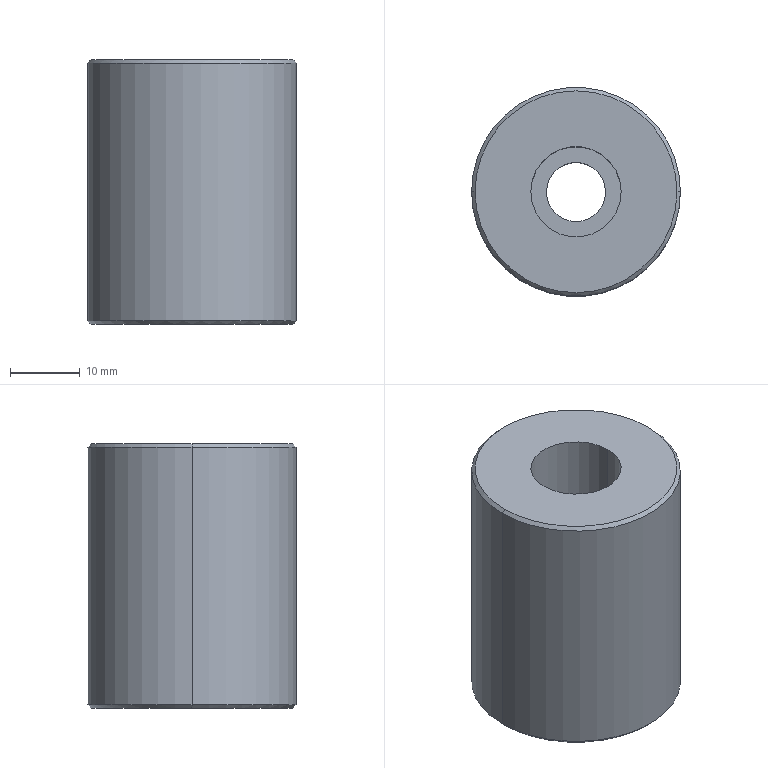Part | STEP file | PN_0003 Press shell nylon post | 1 solid | 13 faces | box 30 x 30 x 38 mm | volume 22857 mm3 | cylinder 6 | cone 4 | plane 3 | commonest cylinder face diameters 8.5 x2 13 x2 30 x2
STEP:
#1=CARTESIAN_POINT('',(0.,0.,0.));
#2=DIRECTION('',(0.,0.,1.));
#3=DIRECTION('',(1.,0.,0.));
#4=AXIS2_PLACEMENT_3D('',#1,#2,#3);
#5=CARTESIAN_POINT('',(14.5,0.,19.));
#6=VERTEX_POINT('',#5);
#7=CARTESIAN_POINT('',(-14.5,0.,19.));
#8=VERTEX_POINT('',#7);
#9=CARTESIAN_POINT('',(0.,0.,19.));
#10=DIRECTION('',(0.,0.,1.));
#11=DIRECTION('',(1.,0.,0.));
#12=AXIS2_PLACEMENT_3D('',#9,#10,#11);
#13=CIRCLE('',#12,14.5);
#14=CARTESIAN_POINT('',(0.,0.,19.));
#15=DIRECTION('',(0.,0.,-1.));
#16=DIRECTION('',(-1.,0.,0.));
#17=AXIS2_PLACEMENT_3D('',#14,#15,#16);
#18=CONICAL_SURFACE('',#17,14.5,0.7854);
#19=CARTESIAN_POINT('',(3.142,0.));
#20=DIRECTION('',(-1.,0.));
#21=VECTOR('',#20,1.);
#22=LINE('',#19,#21);
#23=(GEOMETRIC_REPRESENTATION_CONTEXT(2)PARAMETRIC_REPRESENTATION_CONTEXT()REPRESENTATION_CONTEXT('',''));
#24=DEFINITIONAL_REPRESENTATION('',(#22),#23);
#25=PCURVE('',#18,#24);
#26=CARTESIAN_POINT('',(0.,0.,19.));
#27=DIRECTION('',(0.,0.,1.));
#28=DIRECTION('',(1.,0.,0.));
#29=AXIS2_PLACEMENT_3D('',#26,#27,#28);
#30=PLANE('',#29);
#31=CARTESIAN_POINT('',(0.,0.));
#32=DIRECTION('',(1.,0.));
#33=AXIS2_PLACEMENT_2D('',#31,#32);
#34=CIRCLE('',#33,14.5);
#35=(GEOMETRIC_REPRESENTATION_CONTEXT(2)PARAMETRIC_REPRESENTATION_CONTEXT()REPRESENTATION_CONTEXT('',''));
#36=DEFINITIONAL_REPRESENTATION('',(#34),#35);
#37=PCURVE('',#30,#36);
#38=SURFACE_CURVE('',#13,(#25,#37),.PCURVE_S1.);
#39=EDGE_CURVE('',#6,#8,#38,.T.);
#40=ORIENTED_EDGE('',*,*,#39,.F.);
#41=CARTESIAN_POINT('',(15.,0.,18.5));
#42=VERTEX_POINT('',#41);
#43=CARTESIAN_POINT('',(14.5,0.,19.));
#44=DIRECTION('',(0.7071,0.,-0.7071));
#45=VECTOR('',#44,1.);
#46=LINE('',#43,#45);
#47=CARTESIAN_POINT('',(3.142,0.));
#48=DIRECTION('',(0.,1.));
#49=VECTOR('',#48,1.);
#50=LINE('',#47,#49);
#51=(GEOMETRIC_REPRESENTATION_CONTEXT(2)PARAMETRIC_REPRESENTATION_CONTEXT()REPRESENTATION_CONTEXT('',''));
#52=DEFINITIONAL_REPRESENTATION('',(#50),#51);
#53=PCURVE('',#18,#52);
#54=CARTESIAN_POINT('',(0.,0.,19.));
#55=DIRECTION('',(0.,0.,-1.));
#56=DIRECTION('',(-1.,0.,0.));
#57=AXIS2_PLACEMENT_3D('',#54,#55,#56);
#58=CONICAL_SURFACE('',#57,14.5,0.7854);
#59=CARTESIAN_POINT('',(3.142,0.));
#60=DIRECTION('',(0.,1.));
#61=VECTOR('',#60,1.);
#62=LINE('',#59,#61);
#63=(GEOMETRIC_REPRESENTATION_CONTEXT(2)PARAMETRIC_REPRESENTATION_CONTEXT()REPRESENTATION_CONTEXT('',''));
#64=DEFINITIONAL_REPRESENTATION('',(#62),#63);
#65=PCURVE('',#58,#64);
#66=SURFACE_CURVE('',#46,(#53,#65),.PCURVE_S1.);
#67=EDGE_CURVE('',#6,#42,#66,.T.);
#68=ORIENTED_EDGE('',*,*,#67,.T.);
#69=CARTESIAN_POINT('',(-15.,0.,18.5));
#70=VERTEX_POINT('',#69);
#71=CARTESIAN_POINT('',(0.,0.,18.5));
#72=DIRECTION('',(0.,0.,-1.));
#73=DIRECTION('',(1.,0.,0.));
#74=AXIS2_PLACEMENT_3D('',#71,#72,#73);
#75=CIRCLE('',#74,15.);
#76=CARTESIAN_POINT('',(-3.142,0.5));
#77=DIRECTION('',(1.,0.));
#78=VECTOR('',#77,1.);
#79=LINE('',#76,#78);
#80=(GEOMETRIC_REPRESENTATION_CONTEXT(2)PARAMETRIC_REPRESENTATION_CONTEXT()REPRESENTATION_CONTEXT('',''));
#81=DEFINITIONAL_REPRESENTATION('',(#79),#80);
#82=PCURVE('',#18,#81);
#83=CARTESIAN_POINT('',(0.,0.,19.));
#84=DIRECTION('',(0.,0.,-1.));
#85=DIRECTION('',(-1.,0.,0.));
#86=AXIS2_PLACEMENT_3D('',#83,#84,#85);
#87=CYLINDRICAL_SURFACE('',#86,15.);
#88=CARTESIAN_POINT('',(-3.142,0.5));
#89=DIRECTION('',(1.,0.));
#90=VECTOR('',#89,1.);
#91=LINE('',#88,#90);
#92=(GEOMETRIC_REPRESENTATION_CONTEXT(2)PARAMETRIC_REPRESENTATION_CONTEXT()REPRESENTATION_CONTEXT('',''));
#93=DEFINITIONAL_REPRESENTATION('',(#91),#92);
#94=PCURVE('',#87,#93);
#95=SURFACE_CURVE('',#75,(#82,#94),.PCURVE_S1.);
#96=EDGE_CURVE('',#70,#42,#95,.T.);
#97=ORIENTED_EDGE('',*,*,#96,.F.);
#98=CARTESIAN_POINT('',(-14.5,0.,19.));
#99=DIRECTION('',(-0.7071,0.,-0.7071));
#100=VECTOR('',#99,1.);
#101=LINE('',#98,#100);
#102=CARTESIAN_POINT('',(0.,0.));
#103=DIRECTION('',(0.,1.));
#104=VECTOR('',#103,1.);
#105=LINE('',#102,#104);
#106=(GEOMETRIC_REPRESENTATION_CONTEXT(2)PARAMETRIC_REPRESENTATION_CONTEXT()REPRESENTATION_CONTEXT('',''));
#107=DEFINITIONAL_REPRESENTATION('',(#105),#106);
#108=PCURVE('',#18,#107);
#109=CARTESIAN_POINT('',(6.283,0.));
#110=DIRECTION('',(0.,1.));
#111=VECTOR('',#110,1.);
#112=LINE('',#109,#111);
#113=(GEOMETRIC_REPRESENTATION_CONTEXT(2)PARAMETRIC_REPRESENTATION_CONTEXT()REPRESENTATION_CONTEXT('',''));
#114=DEFINITIONAL_REPRESENTATION('',(#112),#113);
#115=PCURVE('',#58,#114);
#116=SURFACE_CURVE('',#101,(#108,#115),.PCURVE_S1.);
#117=EDGE_CURVE('',#8,#70,#116,.T.);
#118=ORIENTED_EDGE('',*,*,#117,.F.);
#119=EDGE_LOOP('',(#40,#68,#97,#118));
#120=FACE_BOUND('',#119,.T.);
#121=ADVANCED_FACE('',(#120),#18,.T.);
#122=CARTESIAN_POINT('',(-14.5,0.,-19.));
#123=VERTEX_POINT('',#122);
#124=CARTESIAN_POINT('',(14.5,0.,-19.));
#125=VERTEX_POINT('',#124);
#126=CARTESIAN_POINT('',(0.,0.,-19.));
#127=DIRECTION('',(0.,0.,-1.));
#128=DIRECTION('',(1.,0.,0.));
#129=AXIS2_PLACEMENT_3D('',#126,#127,#128);
#130=CIRCLE('',#129,14.5);
#131=CARTESIAN_POINT('',(0.,0.,-18.5));
#132=DIRECTION('',(0.,0.,1.));
#133=DIRECTION('',(1.,0.,0.));
#134=AXIS2_PLACEMENT_3D('',#131,#132,#133);
#135=CONICAL_SURFACE('',#134,15.,0.7854);
#136=CARTESIAN_POINT('',(6.283,-0.5));
#137=DIRECTION('',(-1.,0.));
#138=VECTOR('',#137,1.);
#139=LINE('',#136,#138);
#140=(GEOMETRIC_REPRESENTATION_CONTEXT(2)PARAMETRIC_REPRESENTATION_CONTEXT()REPRESENTATION_CONTEXT('',''));
#141=DEFINITIONAL_REPRESENTATION('',(#139),#140);
#142=PCURVE('',#135,#141);
#143=CARTESIAN_POINT('',(0.,0.,-19.));
#144=DIRECTION('',(0.,0.,1.));
#145=DIRECTION('',(1.,0.,0.));
#146=AXIS2_PLACEMENT_3D('',#143,#144,#145);
#147=PLANE('',#146);
#148=CARTESIAN_POINT('',(14.5,0.));
#149=CARTESIAN_POINT('',(14.5,-25.115));
#150=CARTESIAN_POINT('',(-7.25,-12.557));
#151=CARTESIAN_POINT('',(-29.,0.));
#152=CARTESIAN_POINT('',(-7.25,12.557));
#153=CARTESIAN_POINT('',(14.5,25.115));
#154=CARTESIAN_POINT('',(14.5,0.));
#155=(BOUNDED_CURVE()B_SPLINE_CURVE(2,(#148,#149,#150,#151,#152,#153,#154),.UNSPECIFIED.,.T.,.F.)B_SPLINE_CURVE_WITH_KNOTS((1,2,2,2,2,1),(-2.094,0.,2.094,4.189,6.283,8.378),.UNSPECIFIED.)CURVE()GEOMETRIC_REPRESENTATION_ITEM()RATIONAL_B_SPLINE_CURVE((1.,0.5,1.,0.5,1.,0.5,1.))REPRESENTATION_ITEM(''));
#156=(GEOMETRIC_REPRESENTATION_CONTEXT(2)PARAMETRIC_REPRESENTATION_CONTEXT()REPRESENTATION_CONTEXT('',''));
#157=DEFINITIONAL_REPRESENTATION('',(#155),#156);
#158=PCURVE('',#147,#157);
#159=SURFACE_CURVE('',#130,(#142,#158),.PCURVE_S1.);
#160=EDGE_CURVE('',#123,#125,#159,.T.);
#161=ORIENTED_EDGE('',*,*,#160,.F.);
#162=CARTESIAN_POINT('',(-15.,0.,-18.5));
#163=VERTEX_POINT('',#162);
#164=CARTESIAN_POINT('',(-15.,0.,-18.5));
#165=DIRECTION('',(-0.7071,0.,0.7071));
#166=VECTOR('',#165,1.);
#167=LINE('',#164,#166);
#168=CARTESIAN_POINT('',(3.142,0.));
#169=DIRECTION('',(0.,1.));
#170=VECTOR('',#169,1.);
#171=LINE('',#168,#170);
#172=(GEOMETRIC_REPRESENTATION_CONTEXT(2)PARAMETRIC_REPRESENTATION_CONTEXT()REPRESENTATION_CONTEXT('',''));
#173=DEFINITIONAL_REPRESENTATION('',(#171),#172);
#174=PCURVE('',#135,#173);
#175=CARTESIAN_POINT('',(0.,0.,-18.5));
#176=DIRECTION('',(0.,0.,1.));
#177=DIRECTION('',(1.,0.,0.));
#178=AXIS2_PLACEMENT_3D('',#175,#176,#177);
#179=CONICAL_SURFACE('',#178,15.,0.7854);
#180=CARTESIAN_POINT('',(3.142,0.));
#181=DIRECTION('',(0.,1.));
#182=VECTOR('',#181,1.);
#183=LINE('',#180,#182);
#184=(GEOMETRIC_REPRESENTATION_CONTEXT(2)PARAMETRIC_REPRESENTATION_CONTEXT()REPRESENTATION_CONTEXT('',''));
#185=DEFINITIONAL_REPRESENTATION('',(#183),#184);
#186=PCURVE('',#179,#185);
#187=SURFACE_CURVE('',#167,(#174,#186),.PCURVE_S1.);
#188=EDGE_CURVE('',#123,#163,#187,.T.);
#189=ORIENTED_EDGE('',*,*,#188,.T.);
#190=CARTESIAN_POINT('',(15.,0.,-18.5));
#191=VERTEX_POINT('',#190);
#192=CARTESIAN_POINT('',(0.,0.,-18.5));
#193=DIRECTION('',(0.,0.,1.));
#194=DIRECTION('',(1.,0.,0.));
#195=AXIS2_PLACEMENT_3D('',#192,#193,#194);
#196=CIRCLE('',#195,15.);
#197=CARTESIAN_POINT('',(0.,0.));
#198=DIRECTION('',(1.,0.));
#199=VECTOR('',#198,1.);
#200=LINE('',#197,#199);
#201=(GEOMETRIC_REPRESENTATION_CONTEXT(2)PARAMETRIC_REPRESENTATION_CONTEXT()REPRESENTATION_CONTEXT('',''));
#202=DEFINITIONAL_REPRESENTATION('',(#200),#201);
#203=PCURVE('',#135,#202);
#204=CARTESIAN_POINT('',(3.142,37.5));
#205=DIRECTION('',(-1.,0.));
#206=VECTOR('',#205,1.);
#207=LINE('',#204,#206);
#208=(GEOMETRIC_REPRESENTATION_CONTEXT(2)PARAMETRIC_REPRESENTATION_CONTEXT()REPRESENTATION_CONTEXT('',''));
#209=DEFINITIONAL_REPRESENTATION('',(#207),#208);
#210=PCURVE('',#87,#209);
#211=SURFACE_CURVE('',#196,(#203,#210),.PCURVE_S1.);
#212=EDGE_CURVE('',#191,#163,#211,.T.);
#213=ORIENTED_EDGE('',*,*,#212,.F.);
#214=CARTESIAN_POINT('',(15.,0.,-18.5));
#215=DIRECTION('',(0.7071,0.,0.7071));
#216=VECTOR('',#215,1.);
#217=LINE('',#214,#216);
#218=CARTESIAN_POINT('',(0.,0.));
#219=DIRECTION('',(0.,1.));
#220=VECTOR('',#219,1.);
#221=LINE('',#218,#220);
#222=(GEOMETRIC_REPRESENTATION_CONTEXT(2)PARAMETRIC_REPRESENTATION_CONTEXT()REPRESENTATION_CONTEXT('',''));
#223=DEFINITIONAL_REPRESENTATION('',(#221),#222);
#224=PCURVE('',#135,#223);
#225=CARTESIAN_POINT('',(6.283,0.));
#226=DIRECTION('',(0.,1.));
#227=VECTOR('',#226,1.);
#228=LINE('',#225,#227);
#229=(GEOMETRIC_REPRESENTATION_CONTEXT(2)PARAMETRIC_REPRESENTATION_CONTEXT()REPRESENTATION_CONTEXT('',''));
#230=DEFINITIONAL_REPRESENTATION('',(#228),#229);
#231=PCURVE('',#179,#230);
#232=SURFACE_CURVE('',#217,(#224,#231),.PCURVE_S1.);
#233=EDGE_CURVE('',#125,#191,#232,.T.);
#234=ORIENTED_EDGE('',*,*,#233,.F.);
#235=EDGE_LOOP('',(#161,#189,#213,#234));
#236=FACE_BOUND('',#235,.T.);
#237=ADVANCED_FACE('',(#236),#135,.T.);
#238=CARTESIAN_POINT('',(-4.25,0.,-5.));
#239=VERTEX_POINT('',#238);
#240=CARTESIAN_POINT('',(-4.25,0.,-19.));
#241=VERTEX_POINT('',#240);
#242=CARTESIAN_POINT('',(-4.25,0.,19.));
#243=DIRECTION('',(0.,0.,-1.));
#244=VECTOR('',#243,1.);
#245=LINE('',#242,#244);
#246=CARTESIAN_POINT('',(0.,0.,19.));
#247=DIRECTION('',(0.,0.,-1.));
#248=DIRECTION('',(-1.,0.,0.));
#249=AXIS2_PLACEMENT_3D('',#246,#247,#248);
#250=CYLINDRICAL_SURFACE('',#249,4.25);
#251=CARTESIAN_POINT('',(6.283,0.));
#252=DIRECTION('',(0.,1.));
#253=VECTOR('',#252,1.);
#254=LINE('',#251,#253);
#255=(GEOMETRIC_REPRESENTATION_CONTEXT(2)PARAMETRIC_REPRESENTATION_CONTEXT()REPRESENTATION_CONTEXT('',''));
#256=DEFINITIONAL_REPRESENTATION('',(#254),#255);
#257=PCURVE('',#250,#256);
#258=CARTESIAN_POINT('',(0.,0.,19.));
#259=DIRECTION('',(0.,0.,-1.));
#260=DIRECTION('',(-1.,0.,0.));
#261=AXIS2_PLACEMENT_3D('',#258,#259,#260);
#262=CYLINDRICAL_SURFACE('',#261,4.25);
#263=CARTESIAN_POINT('',(0.,0.));
#264=DIRECTION('',(0.,1.));
#265=VECTOR('',#264,1.);
#266=LINE('',#263,#265);
#267=(GEOMETRIC_REPRESENTATION_CONTEXT(2)PARAMETRIC_REPRESENTATION_CONTEXT()REPRESENTATION_CONTEXT('',''));
#268=DEFINITIONAL_REPRESENTATION('',(#266),#267);
#269=PCURVE('',#262,#268);
#270=SURFACE_CURVE('',#245,(#257,#269),.PCURVE_S1.);
#271=EDGE_CURVE('',#239,#241,#270,.T.);
#272=ORIENTED_EDGE('',*,*,#271,.T.);
#273=CARTESIAN_POINT('',(4.25,0.,-19.));
#274=VERTEX_POINT('',#273);
#275=CARTESIAN_POINT('',(0.,0.,-19.));
#276=DIRECTION('',(0.,0.,-1.));
#277=DIRECTION('',(-1.,0.,0.));
#278=AXIS2_PLACEMENT_3D('',#275,#276,#277);
#279=CIRCLE('',#278,4.25);
#280=CARTESIAN_POINT('',(0.,38.));
#281=DIRECTION('',(1.,0.));
#282=VECTOR('',#281,1.);
#283=LINE('',#280,#282);
#284=(GEOMETRIC_REPRESENTATION_CONTEXT(2)PARAMETRIC_REPRESENTATION_CONTEXT()REPRESENTATION_CONTEXT('',''));
#285=DEFINITIONAL_REPRESENTATION('',(#283),#284);
#286=PCURVE('',#250,#285);
#287=CARTESIAN_POINT('',(-4.25,0.));
#288=CARTESIAN_POINT('',(-4.25,7.361));
#289=CARTESIAN_POINT('',(2.125,3.681));
#290=CARTESIAN_POINT('',(8.5,0.));
#291=CARTESIAN_POINT('',(2.125,-3.681));
#292=CARTESIAN_POINT('',(-4.25,-7.361));
#293=CARTESIAN_POINT('',(-4.25,0.));
#294=(BOUNDED_CURVE()B_SPLINE_CURVE(2,(#287,#288,#289,#290,#291,#292,#293),.UNSPECIFIED.,.T.,.F.)B_SPLINE_CURVE_WITH_KNOTS((1,2,2,2,2,1),(-2.094,0.,2.094,4.189,6.283,8.378),.UNSPECIFIED.)CURVE()GEOMETRIC_REPRESENTATION_ITEM()RATIONAL_B_SPLINE_CURVE((1.,0.5,1.,0.5,1.,0.5,1.))REPRESENTATION_ITEM(''));
#295=(GEOMETRIC_REPRESENTATION_CONTEXT(2)PARAMETRIC_REPRESENTATION_CONTEXT()REPRESENTATION_CONTEXT('',''));
#296=DEFINITIONAL_REPRESENTATION('',(#294),#295);
#297=PCURVE('',#147,#296);
#298=SURFACE_CURVE('',#279,(#286,#297),.PCURVE_S1.);
#299=EDGE_CURVE('',#274,#241,#298,.T.);
#300=ORIENTED_EDGE('',*,*,#299,.F.);
#301=CARTESIAN_POINT('',(4.25,0.,-5.));
#302=VERTEX_POINT('',#301);
#303=CARTESIAN_POINT('',(4.25,0.,19.));
#304=DIRECTION('',(0.,0.,-1.));
#305=VECTOR('',#304,1.);
#306=LINE('',#303,#305);
#307=CARTESIAN_POINT('',(3.142,0.));
#308=DIRECTION('',(0.,1.));
#309=VECTOR('',#308,1.);
#310=LINE('',#307,#309);
#311=(GEOMETRIC_REPRESENTATION_CONTEXT(2)PARAMETRIC_REPRESENTATION_CONTEXT()REPRESENTATION_CONTEXT('',''));
#312=DEFINITIONAL_REPRESENTATION('',(#310),#311);
#313=PCURVE('',#250,#312);
#314=CARTESIAN_POINT('',(3.142,0.));
#315=DIRECTION('',(0.,1.));
#316=VECTOR('',#315,1.);
#317=LINE('',#314,#316);
#318=(GEOMETRIC_REPRESENTATION_CONTEXT(2)PARAMETRIC_REPRESENTATION_CONTEXT()REPRESENTATION_CONTEXT('',''));
#319=DEFINITIONAL_REPRESENTATION('',(#317),#318);
#320=PCURVE('',#262,#319);
#321=SURFACE_CURVE('',#306,(#313,#320),.PCURVE_S1.);
#322=EDGE_CURVE('',#302,#274,#321,.T.);
#323=ORIENTED_EDGE('',*,*,#322,.F.);
#324=CARTESIAN_POINT('',(0.,0.,-5.));
#325=DIRECTION('',(0.,0.,1.));
#326=DIRECTION('',(1.,0.,0.));
#327=AXIS2_PLACEMENT_3D('',#324,#325,#326);
#328=CIRCLE('',#327,4.25);
#329=CARTESIAN_POINT('',(9.425,24.));
#330=DIRECTION('',(-1.,0.));
#331=VECTOR('',#330,1.);
#332=LINE('',#329,#331);
#333=(GEOMETRIC_REPRESENTATION_CONTEXT(2)PARAMETRIC_REPRESENTATION_CONTEXT()REPRESENTATION_CONTEXT('',''));
#334=DEFINITIONAL_REPRESENTATION('',(#332),#333);
#335=PCURVE('',#250,#334);
#336=CARTESIAN_POINT('',(0.,0.,-5.));
#337=DIRECTION('',(0.,0.,1.));
#338=DIRECTION('',(1.,0.,0.));
#339=AXIS2_PLACEMENT_3D('',#336,#337,#338);
#340=PLANE('',#339);
#341=CARTESIAN_POINT('',(0.,0.));
#342=DIRECTION('',(1.,0.));
#343=AXIS2_PLACEMENT_2D('',#341,#342);
#344=CIRCLE('',#343,4.25);
#345=(GEOMETRIC_REPRESENTATION_CONTEXT(2)PARAMETRIC_REPRESENTATION_CONTEXT()REPRESENTATION_CONTEXT('',''));
#346=DEFINITIONAL_REPRESENTATION('',(#344),#345);
#347=PCURVE('',#340,#346);
#348=SURFACE_CURVE('',#328,(#335,#347),.PCURVE_S1.);
#349=EDGE_CURVE('',#239,#302,#348,.T.);
#350=ORIENTED_EDGE('',*,*,#349,.F.);
#351=EDGE_LOOP('',(#272,#300,#323,#350));
#352=FACE_BOUND('',#351,.F.);
#353=ADVANCED_FACE('',(#352),#250,.F.);
#354=CARTESIAN_POINT('',(6.5,0.,-5.));
#355=VERTEX_POINT('',#354);
#356=CARTESIAN_POINT('',(6.5,0.,19.));
#357=VERTEX_POINT('',#356);
#358=CARTESIAN_POINT('',(6.5,0.,-5.));
#359=DIRECTION('',(0.,0.,1.));
#360=VECTOR('',#359,1.);
#361=LINE('',#358,#360);
#362=CARTESIAN_POINT('',(0.,0.,-5.));
#363=DIRECTION('',(0.,0.,1.));
#364=DIRECTION('',(1.,0.,0.));
#365=AXIS2_PLACEMENT_3D('',#362,#363,#364);
#366=CYLINDRICAL_SURFACE('',#365,6.5);
#367=CARTESIAN_POINT('',(6.283,0.));
#368=DIRECTION('',(0.,1.));
#369=VECTOR('',#368,1.);
#370=LINE('',#367,#369);
#371=(GEOMETRIC_REPRESENTATION_CONTEXT(2)PARAMETRIC_REPRESENTATION_CONTEXT()REPRESENTATION_CONTEXT('',''));
#372=DEFINITIONAL_REPRESENTATION('',(#370),#371);
#373=PCURVE('',#366,#372);
#374=CARTESIAN_POINT('',(0.,0.,-5.));
#375=DIRECTION('',(0.,0.,1.));
#376=DIRECTION('',(1.,0.,0.));
#377=AXIS2_PLACEMENT_3D('',#374,#375,#376);
#378=CYLINDRICAL_SURFACE('',#377,6.5);
#379=CARTESIAN_POINT('',(0.,0.));
#380=DIRECTION('',(0.,1.));
#381=VECTOR('',#380,1.);
#382=LINE('',#379,#381);
#383=(GEOMETRIC_REPRESENTATION_CONTEXT(2)PARAMETRIC_REPRESENTATION_CONTEXT()REPRESENTATION_CONTEXT('',''));
#384=DEFINITIONAL_REPRESENTATION('',(#382),#383);
#385=PCURVE('',#378,#384);
#386=SURFACE_CURVE('',#361,(#373,#385),.PCURVE_S1.);
#387=EDGE_CURVE('',#355,#357,#386,.T.);
#388=ORIENTED_EDGE('',*,*,#387,.T.);
#389=CARTESIAN_POINT('',(-6.5,0.,19.));
#390=VERTEX_POINT('',#389);
#391=CARTESIAN_POINT('',(0.,0.,19.));
#392=DIRECTION('',(0.,0.,1.));
#393=DIRECTION('',(1.,0.,0.));
#394=AXIS2_PLACEMENT_3D('',#391,#392,#393);
#395=CIRCLE('',#394,6.5);
#396=CARTESIAN_POINT('',(0.,24.));
#397=DIRECTION('',(1.,0.));
#398=VECTOR('',#397,1.);
#399=LINE('',#396,#398);
#400=(GEOMETRIC_REPRESENTATION_CONTEXT(2)PARAMETRIC_REPRESENTATION_CONTEXT()REPRESENTATION_CONTEXT('',''));
#401=DEFINITIONAL_REPRESENTATION('',(#399),#400);
#402=PCURVE('',#366,#401);
#403=CARTESIAN_POINT('',(0.,0.));
#404=DIRECTION('',(1.,0.));
#405=AXIS2_PLACEMENT_2D('',#403,#404);
#406=CIRCLE('',#405,6.5);
#407=(GEOMETRIC_REPRESENTATION_CONTEXT(2)PARAMETRIC_REPRESENTATION_CONTEXT()REPRESENTATION_CONTEXT('',''));
#408=DEFINITIONAL_REPRESENTATION('',(#406),#407);
#409=PCURVE('',#30,#408);
#410=SURFACE_CURVE('',#395,(#402,#409),.PCURVE_S1.);
#411=EDGE_CURVE('',#390,#357,#410,.T.);
#412=ORIENTED_EDGE('',*,*,#411,.F.);
#413=CARTESIAN_POINT('',(-6.5,0.,-5.));
#414=VERTEX_POINT('',#413);
#415=CARTESIAN_POINT('',(-6.5,0.,-5.));
#416=DIRECTION('',(0.,0.,1.));
#417=VECTOR('',#416,1.);
#418=LINE('',#415,#417);
#419=CARTESIAN_POINT('',(3.142,0.));
#420=DIRECTION('',(0.,1.));
#421=VECTOR('',#420,1.);
#422=LINE('',#419,#421);
#423=(GEOMETRIC_REPRESENTATION_CONTEXT(2)PARAMETRIC_REPRESENTATION_CONTEXT()REPRESENTATION_CONTEXT('',''));
#424=DEFINITIONAL_REPRESENTATION('',(#422),#423);
#425=PCURVE('',#366,#424);
#426=CARTESIAN_POINT('',(3.142,0.));
#427=DIRECTION('',(0.,1.));
#428=VECTOR('',#427,1.);
#429=LINE('',#426,#428);
#430=(GEOMETRIC_REPRESENTATION_CONTEXT(2)PARAMETRIC_REPRESENTATION_CONTEXT()REPRESENTATION_CONTEXT('',''));
#431=DEFINITIONAL_REPRESENTATION('',(#429),#430);
#432=PCURVE('',#378,#431);
#433=SURFACE_CURVE('',#418,(#425,#432),.PCURVE_S1.);
#434=EDGE_CURVE('',#414,#390,#433,.T.);
#435=ORIENTED_EDGE('',*,*,#434,.F.);
#436=CARTESIAN_POINT('',(0.,0.,-5.));
#437=DIRECTION('',(0.,0.,1.));
#438=DIRECTION('',(1.,0.,0.));
#439=AXIS2_PLACEMENT_3D('',#436,#437,#438);
#440=CIRCLE('',#439,6.5);
#441=CARTESIAN_POINT('',(0.,0.));
#442=DIRECTION('',(1.,0.));
#443=VECTOR('',#442,1.);
#444=LINE('',#441,#443);
#445=(GEOMETRIC_REPRESENTATION_CONTEXT(2)PARAMETRIC_REPRESENTATION_CONTEXT()REPRESENTATION_CONTEXT('',''));
#446=DEFINITIONAL_REPRESENTATION('',(#444),#445);
#447=PCURVE('',#366,#446);
#448=CARTESIAN_POINT('',(0.,0.));
#449=DIRECTION('',(1.,0.));
#450=AXIS2_PLACEMENT_2D('',#448,#449);
#451=CIRCLE('',#450,6.5);
#452=(GEOMETRIC_REPRESENTATION_CONTEXT(2)PARAMETRIC_REPRESENTATION_CONTEXT()REPRESENTATION_CONTEXT('',''));
#453=DEFINITIONAL_REPRESENTATION('',(#451),#452);
#454=PCURVE('',#340,#453);
#455=SURFACE_CURVE('',#440,(#447,#454),.PCURVE_S1.);
#456=EDGE_CURVE('',#414,#355,#455,.T.);
#457=ORIENTED_EDGE('',*,*,#456,.T.);
#458=EDGE_LOOP('',(#388,#412,#435,#457));
#459=FACE_BOUND('',#458,.F.);
#460=ADVANCED_FACE('',(#459),#366,.F.);
#461=ORIENTED_EDGE('',*,*,#96,.T.);
#462=CARTESIAN_POINT('',(15.,0.,19.));
#463=DIRECTION('',(0.,0.,-1.));
#464=VECTOR('',#463,1.);
#465=LINE('',#462,#464);
#466=CARTESIAN_POINT('',(3.142,0.));
#467=DIRECTION('',(0.,1.));
#468=VECTOR('',#467,1.);
#469=LINE('',#466,#468);
#470=(GEOMETRIC_REPRESENTATION_CONTEXT(2)PARAMETRIC_REPRESENTATION_CONTEXT()REPRESENTATION_CONTEXT('',''));
#471=DEFINITIONAL_REPRESENTATION('',(#469),#470);
#472=PCURVE('',#87,#471);
#473=CARTESIAN_POINT('',(0.,0.,19.));
#474=DIRECTION('',(0.,0.,-1.));
#475=DIRECTION('',(-1.,0.,0.));
#476=AXIS2_PLACEMENT_3D('',#473,#474,#475);
#477=CYLINDRICAL_SURFACE('',#476,15.);
#478=CARTESIAN_POINT('',(3.142,0.));
#479=DIRECTION('',(0.,1.));
#480=VECTOR('',#479,1.);
#481=LINE('',#478,#480);
#482=(GEOMETRIC_REPRESENTATION_CONTEXT(2)PARAMETRIC_REPRESENTATION_CONTEXT()REPRESENTATION_CONTEXT('',''));
#483=DEFINITIONAL_REPRESENTATION('',(#481),#482);
#484=PCURVE('',#477,#483);
#485=SURFACE_CURVE('',#465,(#472,#484),.PCURVE_S1.);
#486=EDGE_CURVE('',#42,#191,#485,.T.);
#487=ORIENTED_EDGE('',*,*,#486,.T.);
#488=ORIENTED_EDGE('',*,*,#212,.T.);
#489=CARTESIAN_POINT('',(-15.,0.,19.));
#490=DIRECTION('',(0.,0.,-1.));
#491=VECTOR('',#490,1.);
#492=LINE('',#489,#491);
#493=CARTESIAN_POINT('',(0.,0.));
#494=DIRECTION('',(0.,1.));
#495=VECTOR('',#494,1.);
#496=LINE('',#493,#495);
#497=(GEOMETRIC_REPRESENTATION_CONTEXT(2)PARAMETRIC_REPRESENTATION_CONTEXT()REPRESENTATION_CONTEXT('',''));
#498=DEFINITIONAL_REPRESENTATION('',(#496),#497);
#499=PCURVE('',#87,#498);
#500=CARTESIAN_POINT('',(6.283,0.));
#501=DIRECTION('',(0.,1.));
#502=VECTOR('',#501,1.);
#503=LINE('',#500,#502);
#504=(GEOMETRIC_REPRESENTATION_CONTEXT(2)PARAMETRIC_REPRESENTATION_CONTEXT()REPRESENTATION_CONTEXT('',''));
#505=DEFINITIONAL_REPRESENTATION('',(#503),#504);
#506=PCURVE('',#477,#505);
#507=SURFACE_CURVE('',#492,(#499,#506),.PCURVE_S1.);
#508=EDGE_CURVE('',#70,#163,#507,.T.);
#509=ORIENTED_EDGE('',*,*,#508,.F.);
#510=EDGE_LOOP('',(#461,#487,#488,#509));
#511=FACE_BOUND('',#510,.T.);
#512=ADVANCED_FACE('',(#511),#87,.T.);
#513=ORIENTED_EDGE('',*,*,#486,.F.);
#514=CARTESIAN_POINT('',(0.,0.,18.5));
#515=DIRECTION('',(0.,0.,-1.));
#516=DIRECTION('',(1.,0.,0.));
#517=AXIS2_PLACEMENT_3D('',#514,#515,#516);
#518=CIRCLE('',#517,15.);
#519=CARTESIAN_POINT('',(3.142,0.5));
#520=DIRECTION('',(1.,0.));
#521=VECTOR('',#520,1.);
#522=LINE('',#519,#521);
#523=(GEOMETRIC_REPRESENTATION_CONTEXT(2)PARAMETRIC_REPRESENTATION_CONTEXT()REPRESENTATION_CONTEXT('',''));
#524=DEFINITIONAL_REPRESENTATION('',(#522),#523);
#525=PCURVE('',#477,#524);
#526=CARTESIAN_POINT('',(3.142,0.5));
#527=DIRECTION('',(1.,0.));
#528=VECTOR('',#527,1.);
#529=LINE('',#526,#528);
#530=(GEOMETRIC_REPRESENTATION_CONTEXT(2)PARAMETRIC_REPRESENTATION_CONTEXT()REPRESENTATION_CONTEXT('',''));
#531=DEFINITIONAL_REPRESENTATION('',(#529),#530);
#532=PCURVE('',#58,#531);
#533=SURFACE_CURVE('',#518,(#525,#532),.PCURVE_S1.);
#534=EDGE_CURVE('',#42,#70,#533,.T.);
#535=ORIENTED_EDGE('',*,*,#534,.T.);
#536=ORIENTED_EDGE('',*,*,#508,.T.);
#537=CARTESIAN_POINT('',(0.,0.,-18.5));
#538=DIRECTION('',(0.,0.,1.));
#539=DIRECTION('',(1.,0.,0.));
#540=AXIS2_PLACEMENT_3D('',#537,#538,#539);
#541=CIRCLE('',#540,15.);
#542=CARTESIAN_POINT('',(9.425,37.5));
#543=DIRECTION('',(-1.,0.));
#544=VECTOR('',#543,1.);
#545=LINE('',#542,#544);
#546=(GEOMETRIC_REPRESENTATION_CONTEXT(2)PARAMETRIC_REPRESENTATION_CONTEXT()REPRESENTATION_CONTEXT('',''));
#547=DEFINITIONAL_REPRESENTATION('',(#545),#546);
#548=PCURVE('',#477,#547);
#549=CARTESIAN_POINT('',(0.,0.));
#550=DIRECTION('',(1.,0.));
#551=VECTOR('',#550,1.);
#552=LINE('',#549,#551);
#553=(GEOMETRIC_REPRESENTATION_CONTEXT(2)PARAMETRIC_REPRESENTATION_CONTEXT()REPRESENTATION_CONTEXT('',''));
#554=DEFINITIONAL_REPRESENTATION('',(#552),#553);
#555=PCURVE('',#179,#554);
#556=SURFACE_CURVE('',#541,(#548,#555),.PCURVE_S1.);
#557=EDGE_CURVE('',#163,#191,#556,.T.);
#558=ORIENTED_EDGE('',*,*,#557,.T.);
#559=EDGE_LOOP('',(#513,#535,#536,#558));
#560=FACE_BOUND('',#559,.T.);
#561=ADVANCED_FACE('',(#560),#477,.T.);
#562=CARTESIAN_POINT('',(0.,0.,19.));
#563=DIRECTION('',(0.,0.,1.));
#564=DIRECTION('',(1.,0.,0.));
#565=AXIS2_PLACEMENT_3D('',#562,#563,#564);
#566=CIRCLE('',#565,14.5);
#567=CARTESIAN_POINT('',(0.,0.));
#568=DIRECTION('',(1.,0.));
#569=AXIS2_PLACEMENT_2D('',#567,#568);
#570=CIRCLE('',#569,14.5);
#571=(GEOMETRIC_REPRESENTATION_CONTEXT(2)PARAMETRIC_REPRESENTATION_CONTEXT()REPRESENTATION_CONTEXT('',''));
#572=DEFINITIONAL_REPRESENTATION('',(#570),#571);
#573=PCURVE('',#30,#572);
#574=CARTESIAN_POINT('',(9.425,0.));
#575=DIRECTION('',(-1.,0.));
#576=VECTOR('',#575,1.);
#577=LINE('',#574,#576);
#578=(GEOMETRIC_REPRESENTATION_CONTEXT(2)PARAMETRIC_REPRESENTATION_CONTEXT()REPRESENTATION_CONTEXT('',''));
#579=DEFINITIONAL_REPRESENTATION('',(#577),#578);
#580=PCURVE('',#58,#579);
#581=SURFACE_CURVE('',#566,(#573,#580),.PCURVE_S1.);
#582=EDGE_CURVE('',#8,#6,#581,.T.);
#583=ORIENTED_EDGE('',*,*,#582,.T.);
#584=ORIENTED_EDGE('',*,*,#39,.T.);
#585=EDGE_LOOP('',(#583,#584));
#586=FACE_BOUND('',#585,.T.);
#587=CARTESIAN_POINT('',(0.,0.,19.));
#588=DIRECTION('',(0.,0.,1.));
#589=DIRECTION('',(1.,0.,0.));
#590=AXIS2_PLACEMENT_3D('',#587,#588,#589);
#591=CIRCLE('',#590,6.5);
#592=CARTESIAN_POINT('',(0.,0.));
#593=DIRECTION('',(1.,0.));
#594=AXIS2_PLACEMENT_2D('',#592,#593);
#595=CIRCLE('',#594,6.5);
#596=(GEOMETRIC_REPRESENTATION_CONTEXT(2)PARAMETRIC_REPRESENTATION_CONTEXT()REPRESENTATION_CONTEXT('',''));
#597=DEFINITIONAL_REPRESENTATION('',(#595),#596);
#598=PCURVE('',#30,#597);
#599=CARTESIAN_POINT('',(0.,24.));
#600=DIRECTION('',(1.,0.));
#601=VECTOR('',#600,1.);
#602=LINE('',#599,#601);
#603=(GEOMETRIC_REPRESENTATION_CONTEXT(2)PARAMETRIC_REPRESENTATION_CONTEXT()REPRESENTATION_CONTEXT('',''));
#604=DEFINITIONAL_REPRESENTATION('',(#602),#603);
#605=PCURVE('',#378,#604);
#606=SURFACE_CURVE('',#591,(#598,#605),.PCURVE_S1.);
#607=EDGE_CURVE('',#357,#390,#606,.T.);
#608=ORIENTED_EDGE('',*,*,#607,.F.);
#609=ORIENTED_EDGE('',*,*,#411,.F.);
#610=EDGE_LOOP('',(#608,#609));
#611=FACE_BOUND('',#610,.T.);
#612=ADVANCED_FACE('',(#586,#611),#30,.T.);
#613=CARTESIAN_POINT('',(0.,0.,-19.));
#614=DIRECTION('',(0.,0.,-1.));
#615=DIRECTION('',(1.,0.,0.));
#616=AXIS2_PLACEMENT_3D('',#613,#614,#615);
#617=CIRCLE('',#616,14.5);
#618=CARTESIAN_POINT('',(14.5,0.));
#619=CARTESIAN_POINT('',(14.5,-25.115));
#620=CARTESIAN_POINT('',(-7.25,-12.557));
#621=CARTESIAN_POINT('',(-29.,0.));
#622=CARTESIAN_POINT('',(-7.25,12.557));
#623=CARTESIAN_POINT('',(14.5,25.115));
#624=CARTESIAN_POINT('',(14.5,0.));
#625=(BOUNDED_CURVE()B_SPLINE_CURVE(2,(#618,#619,#620,#621,#622,#623,#624),.UNSPECIFIED.,.T.,.F.)B_SPLINE_CURVE_WITH_KNOTS((1,2,2,2,2,1),(-2.094,0.,2.094,4.189,6.283,8.378),.UNSPECIFIED.)CURVE()GEOMETRIC_REPRESENTATION_ITEM()RATIONAL_B_SPLINE_CURVE((1.,0.5,1.,0.5,1.,0.5,1.))REPRESENTATION_ITEM(''));
#626=(GEOMETRIC_REPRESENTATION_CONTEXT(2)PARAMETRIC_REPRESENTATION_CONTEXT()REPRESENTATION_CONTEXT('',''));
#627=DEFINITIONAL_REPRESENTATION('',(#625),#626);
#628=PCURVE('',#147,#627);
#629=CARTESIAN_POINT('',(6.283,-0.5));
#630=DIRECTION('',(-1.,0.));
#631=VECTOR('',#630,1.);
#632=LINE('',#629,#631);
#633=(GEOMETRIC_REPRESENTATION_CONTEXT(2)PARAMETRIC_REPRESENTATION_CONTEXT()REPRESENTATION_CONTEXT('',''));
#634=DEFINITIONAL_REPRESENTATION('',(#632),#633);
#635=PCURVE('',#179,#634);
#636=SURFACE_CURVE('',#617,(#628,#635),.PCURVE_S1.);
#637=EDGE_CURVE('',#125,#123,#636,.T.);
#638=ORIENTED_EDGE('',*,*,#637,.T.);
#639=ORIENTED_EDGE('',*,*,#160,.T.);
#640=EDGE_LOOP('',(#638,#639));
#641=FACE_BOUND('',#640,.T.);
#642=CARTESIAN_POINT('',(0.,0.,-19.));
#643=DIRECTION('',(0.,0.,-1.));
#644=DIRECTION('',(-1.,0.,0.));
#645=AXIS2_PLACEMENT_3D('',#642,#643,#644);
#646=CIRCLE('',#645,4.25);
#647=CARTESIAN_POINT('',(-4.25,0.));
#648=CARTESIAN_POINT('',(-4.25,7.361));
#649=CARTESIAN_POINT('',(2.125,3.681));
#650=CARTESIAN_POINT('',(8.5,0.));
#651=CARTESIAN_POINT('',(2.125,-3.681));
#652=CARTESIAN_POINT('',(-4.25,-7.361));
#653=CARTESIAN_POINT('',(-4.25,0.));
#654=(BOUNDED_CURVE()B_SPLINE_CURVE(2,(#647,#648,#649,#650,#651,#652,#653),.UNSPECIFIED.,.T.,.F.)B_SPLINE_CURVE_WITH_KNOTS((1,2,2,2,2,1),(-2.094,0.,2.094,4.189,6.283,8.378),.UNSPECIFIED.)CURVE()GEOMETRIC_REPRESENTATION_ITEM()RATIONAL_B_SPLINE_CURVE((1.,0.5,1.,0.5,1.,0.5,1.))REPRESENTATION_ITEM(''));
#655=(GEOMETRIC_REPRESENTATION_CONTEXT(2)PARAMETRIC_REPRESENTATION_CONTEXT()REPRESENTATION_CONTEXT('',''));
#656=DEFINITIONAL_REPRESENTATION('',(#654),#655);
#657=PCURVE('',#147,#656);
#658=CARTESIAN_POINT('',(0.,38.));
#659=DIRECTION('',(1.,0.));
#660=VECTOR('',#659,1.);
#661=LINE('',#658,#660);
#662=(GEOMETRIC_REPRESENTATION_CONTEXT(2)PARAMETRIC_REPRESENTATION_CONTEXT()REPRESENTATION_CONTEXT('',''));
#663=DEFINITIONAL_REPRESENTATION('',(#661),#662);
#664=PCURVE('',#262,#663);
#665=SURFACE_CURVE('',#646,(#657,#664),.PCURVE_S1.);
#666=EDGE_CURVE('',#241,#274,#665,.T.);
#667=ORIENTED_EDGE('',*,*,#666,.F.);
#668=ORIENTED_EDGE('',*,*,#299,.F.);
#669=EDGE_LOOP('',(#667,#668));
#670=FACE_BOUND('',#669,.T.);
#671=ADVANCED_FACE('',(#641,#670),#147,.F.);
#672=ORIENTED_EDGE('',*,*,#607,.F.);
#673=ORIENTED_EDGE('',*,*,#387,.F.);
#674=CARTESIAN_POINT('',(0.,0.,-5.));
#675=DIRECTION('',(0.,0.,1.));
#676=DIRECTION('',(1.,0.,0.));
#677=AXIS2_PLACEMENT_3D('',#674,#675,#676);
#678=CIRCLE('',#677,6.5);
#679=CARTESIAN_POINT('',(0.,0.));
#680=DIRECTION('',(1.,0.));
#681=VECTOR('',#680,1.);
#682=LINE('',#679,#681);
#683=(GEOMETRIC_REPRESENTATION_CONTEXT(2)PARAMETRIC_REPRESENTATION_CONTEXT()REPRESENTATION_CONTEXT('',''));
#684=DEFINITIONAL_REPRESENTATION('',(#682),#683);
#685=PCURVE('',#378,#684);
#686=CARTESIAN_POINT('',(0.,0.));
#687=DIRECTION('',(1.,0.));
#688=AXIS2_PLACEMENT_2D('',#686,#687);
#689=CIRCLE('',#688,6.5);
#690=(GEOMETRIC_REPRESENTATION_CONTEXT(2)PARAMETRIC_REPRESENTATION_CONTEXT()REPRESENTATION_CONTEXT('',''));
#691=DEFINITIONAL_REPRESENTATION('',(#689),#690);
#692=PCURVE('',#340,#691);
#693=SURFACE_CURVE('',#678,(#685,#692),.PCURVE_S1.);
#694=EDGE_CURVE('',#355,#414,#693,.T.);
#695=ORIENTED_EDGE('',*,*,#694,.T.);
#696=ORIENTED_EDGE('',*,*,#434,.T.);
#697=EDGE_LOOP('',(#672,#673,#695,#696));
#698=FACE_BOUND('',#697,.F.);
#699=ADVANCED_FACE('',(#698),#378,.F.);
#700=ORIENTED_EDGE('',*,*,#349,.F.);
#701=CARTESIAN_POINT('',(0.,0.,-5.));
#702=DIRECTION('',(0.,0.,1.));
#703=DIRECTION('',(1.,0.,0.));
#704=AXIS2_PLACEMENT_3D('',#701,#702,#703);
#705=CIRCLE('',#704,4.25);
#706=CARTESIAN_POINT('',(0.,0.));
#707=DIRECTION('',(1.,0.));
#708=AXIS2_PLACEMENT_2D('',#706,#707);
#709=CIRCLE('',#708,4.25);
#710=(GEOMETRIC_REPRESENTATION_CONTEXT(2)PARAMETRIC_REPRESENTATION_CONTEXT()REPRESENTATION_CONTEXT('',''));
#711=DEFINITIONAL_REPRESENTATION('',(#709),#710);
#712=PCURVE('',#340,#711);
#713=CARTESIAN_POINT('',(3.142,24.));
#714=DIRECTION('',(-1.,0.));
#715=VECTOR('',#714,1.);
#716=LINE('',#713,#715);
#717=(GEOMETRIC_REPRESENTATION_CONTEXT(2)PARAMETRIC_REPRESENTATION_CONTEXT()REPRESENTATION_CONTEXT('',''));
#718=DEFINITIONAL_REPRESENTATION('',(#716),#717);
#719=PCURVE('',#262,#718);
#720=SURFACE_CURVE('',#705,(#712,#719),.PCURVE_S1.);
#721=EDGE_CURVE('',#302,#239,#720,.T.);
#722=ORIENTED_EDGE('',*,*,#721,.F.);
#723=EDGE_LOOP('',(#700,#722));
#724=FACE_BOUND('',#723,.T.);
#725=ORIENTED_EDGE('',*,*,#694,.T.);
#726=ORIENTED_EDGE('',*,*,#456,.T.);
#727=EDGE_LOOP('',(#725,#726));
#728=FACE_BOUND('',#727,.T.);
#729=ADVANCED_FACE('',(#724,#728),#340,.T.);
#730=ORIENTED_EDGE('',*,*,#666,.F.);
#731=ORIENTED_EDGE('',*,*,#271,.F.);
#732=ORIENTED_EDGE('',*,*,#721,.F.);
#733=ORIENTED_EDGE('',*,*,#322,.T.);
#734=EDGE_LOOP('',(#730,#731,#732,#733));
#735=FACE_BOUND('',#734,.F.);
#736=ADVANCED_FACE('',(#735),#262,.F.);
#737=ORIENTED_EDGE('',*,*,#188,.F.);
#738=ORIENTED_EDGE('',*,*,#637,.F.);
#739=ORIENTED_EDGE('',*,*,#233,.T.);
#740=ORIENTED_EDGE('',*,*,#557,.F.);
#741=EDGE_LOOP('',(#737,#738,#739,#740));
#742=FACE_BOUND('',#741,.T.);
#743=ADVANCED_FACE('',(#742),#179,.T.);
#744=ORIENTED_EDGE('',*,*,#67,.F.);
#745=ORIENTED_EDGE('',*,*,#582,.F.);
#746=ORIENTED_EDGE('',*,*,#117,.T.);
#747=ORIENTED_EDGE('',*,*,#534,.F.);
#748=EDGE_LOOP('',(#744,#745,#746,#747));
#749=FACE_BOUND('',#748,.T.);
#750=ADVANCED_FACE('',(#749),#58,.T.);
#751=CLOSED_SHELL('',(#121,#237,#353,#460,#512,#561,#612,#671,#699,#729,#736,#743,#750));
#752=MANIFOLD_SOLID_BREP('',#751);
#753=(LENGTH_UNIT()NAMED_UNIT(*)SI_UNIT(.MILLI.,.METRE.));
#754=UNCERTAINTY_MEASURE_WITH_UNIT(LENGTH_MEASURE(0.0000001),#753,'','');
#755=(NAMED_UNIT(*)PLANE_ANGLE_UNIT()SI_UNIT($,.RADIAN.));
#756=(NAMED_UNIT(*)SI_UNIT($,.STERADIAN.)SOLID_ANGLE_UNIT());
#757=(GEOMETRIC_REPRESENTATION_CONTEXT(3)GLOBAL_UNCERTAINTY_ASSIGNED_CONTEXT((#754))GLOBAL_UNIT_ASSIGNED_CONTEXT((#753,#755,#756))REPRESENTATION_CONTEXT('',''));
#758=ADVANCED_BREP_SHAPE_REPRESENTATION('',(#4,#752),#757);